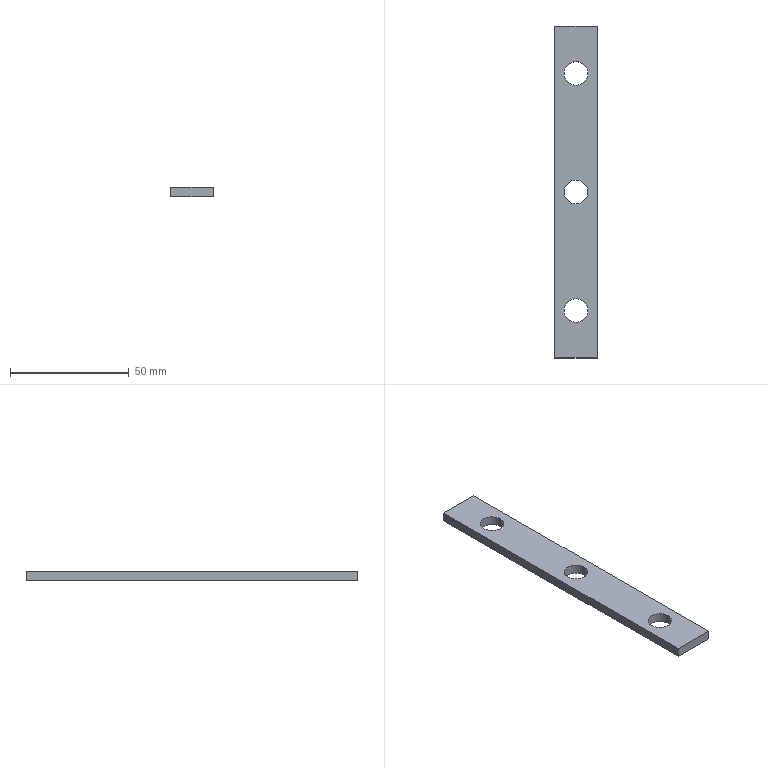Part | SolidWorks | features Extrusion 1 | 1 solid | 12 faces | box 18 x 140 x 4 mm | volume 9138 mm3 | cylinder 6 | plane 6 | commonest cylinder face diameters 10 x6
STEP:
#1=CARTESIAN_POINT('',(-5.,-50.,4.));
#2=VERTEX_POINT('',#1);
#3=CARTESIAN_POINT('',(5.,-50.,4.));
#4=VERTEX_POINT('',#3);
#5=CARTESIAN_POINT('',(0.,-50.,4.));
#6=DIRECTION('',(0.,0.,1.));
#7=DIRECTION('',(1.,0.,0.));
#8=AXIS2_PLACEMENT_3D('',#5,#6,#7);
#9=CIRCLE('',#8,5.);
#10=EDGE_CURVE('',#2,#4,#9,.T.);
#11=ORIENTED_EDGE('',*,*,#10,.T.);
#12=CARTESIAN_POINT('',(5.,-50.,0.));
#13=VERTEX_POINT('',#12);
#14=CARTESIAN_POINT('',(5.,-50.,4.));
#15=DIRECTION('',(0.,0.,-1.));
#16=VECTOR('',#15,1000.);
#17=LINE('',#14,#16);
#18=EDGE_CURVE('',#4,#13,#17,.T.);
#19=ORIENTED_EDGE('',*,*,#18,.T.);
#20=CARTESIAN_POINT('',(-5.,-50.,0.));
#21=VERTEX_POINT('',#20);
#22=CARTESIAN_POINT('',(0.,-50.,0.));
#23=DIRECTION('',(0.,0.,1.));
#24=DIRECTION('',(1.,0.,0.));
#25=AXIS2_PLACEMENT_3D('',#22,#23,#24);
#26=CIRCLE('',#25,5.);
#27=EDGE_CURVE('',#21,#13,#26,.T.);
#28=ORIENTED_EDGE('',*,*,#27,.F.);
#29=CARTESIAN_POINT('',(-5.,-50.,4.));
#30=DIRECTION('',(0.,0.,-1.));
#31=VECTOR('',#30,1000.);
#32=LINE('',#29,#31);
#33=EDGE_CURVE('',#2,#21,#32,.T.);
#34=ORIENTED_EDGE('',*,*,#33,.F.);
#35=EDGE_LOOP('',(#11,#19,#28,#34));
#36=FACE_OUTER_BOUND('',#35,.T.);
#37=CARTESIAN_POINT('',(0.,-50.,4.));
#38=DIRECTION('',(0.,0.,-1.));
#39=DIRECTION('',(-1.,0.,0.));
#40=AXIS2_PLACEMENT_3D('',#37,#38,#39);
#41=CYLINDRICAL_SURFACE('',#40,5.);
#42=ADVANCED_FACE('',(#36),#41,.F.);
#43=CARTESIAN_POINT('',(-5.,0.,4.));
#44=VERTEX_POINT('',#43);
#45=CARTESIAN_POINT('',(5.,0.,4.));
#46=VERTEX_POINT('',#45);
#47=CARTESIAN_POINT('',(0.,0.,4.));
#48=DIRECTION('',(0.,0.,1.));
#49=DIRECTION('',(1.,0.,0.));
#50=AXIS2_PLACEMENT_3D('',#47,#48,#49);
#51=CIRCLE('',#50,5.);
#52=EDGE_CURVE('',#44,#46,#51,.T.);
#53=ORIENTED_EDGE('',*,*,#52,.T.);
#54=CARTESIAN_POINT('',(5.,0.,0.));
#55=VERTEX_POINT('',#54);
#56=CARTESIAN_POINT('',(5.,0.,4.));
#57=DIRECTION('',(0.,0.,-1.));
#58=VECTOR('',#57,1000.);
#59=LINE('',#56,#58);
#60=EDGE_CURVE('',#46,#55,#59,.T.);
#61=ORIENTED_EDGE('',*,*,#60,.T.);
#62=CARTESIAN_POINT('',(-5.,0.,0.));
#63=VERTEX_POINT('',#62);
#64=CARTESIAN_POINT('',(0.,0.,0.));
#65=DIRECTION('',(0.,0.,1.));
#66=DIRECTION('',(1.,0.,0.));
#67=AXIS2_PLACEMENT_3D('',#64,#65,#66);
#68=CIRCLE('',#67,5.);
#69=EDGE_CURVE('',#63,#55,#68,.T.);
#70=ORIENTED_EDGE('',*,*,#69,.F.);
#71=CARTESIAN_POINT('',(-5.,0.,4.));
#72=DIRECTION('',(0.,0.,-1.));
#73=VECTOR('',#72,1000.);
#74=LINE('',#71,#73);
#75=EDGE_CURVE('',#44,#63,#74,.T.);
#76=ORIENTED_EDGE('',*,*,#75,.F.);
#77=EDGE_LOOP('',(#53,#61,#70,#76));
#78=FACE_OUTER_BOUND('',#77,.T.);
#79=CARTESIAN_POINT('',(0.,0.,4.));
#80=DIRECTION('',(0.,0.,-1.));
#81=DIRECTION('',(-1.,0.,0.));
#82=AXIS2_PLACEMENT_3D('',#79,#80,#81);
#83=CYLINDRICAL_SURFACE('',#82,5.);
#84=ADVANCED_FACE('',(#78),#83,.F.);
#85=CARTESIAN_POINT('',(-5.,50.,4.));
#86=VERTEX_POINT('',#85);
#87=CARTESIAN_POINT('',(5.,50.,4.));
#88=VERTEX_POINT('',#87);
#89=CARTESIAN_POINT('',(0.,50.,4.));
#90=DIRECTION('',(0.,0.,1.));
#91=DIRECTION('',(1.,0.,0.));
#92=AXIS2_PLACEMENT_3D('',#89,#90,#91);
#93=CIRCLE('',#92,5.);
#94=EDGE_CURVE('',#86,#88,#93,.T.);
#95=ORIENTED_EDGE('',*,*,#94,.T.);
#96=CARTESIAN_POINT('',(5.,50.,0.));
#97=VERTEX_POINT('',#96);
#98=CARTESIAN_POINT('',(5.,50.,4.));
#99=DIRECTION('',(0.,0.,-1.));
#100=VECTOR('',#99,1000.);
#101=LINE('',#98,#100);
#102=EDGE_CURVE('',#88,#97,#101,.T.);
#103=ORIENTED_EDGE('',*,*,#102,.T.);
#104=CARTESIAN_POINT('',(-5.,50.,0.));
#105=VERTEX_POINT('',#104);
#106=CARTESIAN_POINT('',(0.,50.,0.));
#107=DIRECTION('',(0.,0.,1.));
#108=DIRECTION('',(1.,0.,0.));
#109=AXIS2_PLACEMENT_3D('',#106,#107,#108);
#110=CIRCLE('',#109,5.);
#111=EDGE_CURVE('',#105,#97,#110,.T.);
#112=ORIENTED_EDGE('',*,*,#111,.F.);
#113=CARTESIAN_POINT('',(-5.,50.,4.));
#114=DIRECTION('',(0.,0.,-1.));
#115=VECTOR('',#114,1000.);
#116=LINE('',#113,#115);
#117=EDGE_CURVE('',#86,#105,#116,.T.);
#118=ORIENTED_EDGE('',*,*,#117,.F.);
#119=EDGE_LOOP('',(#95,#103,#112,#118));
#120=FACE_OUTER_BOUND('',#119,.T.);
#121=CARTESIAN_POINT('',(0.,50.,4.));
#122=DIRECTION('',(0.,0.,-1.));
#123=DIRECTION('',(-1.,0.,0.));
#124=AXIS2_PLACEMENT_3D('',#121,#122,#123);
#125=CYLINDRICAL_SURFACE('',#124,5.);
#126=ADVANCED_FACE('',(#120),#125,.F.);
#127=CARTESIAN_POINT('',(9.,-70.,4.));
#128=VERTEX_POINT('',#127);
#129=CARTESIAN_POINT('',(9.,70.,4.));
#130=VERTEX_POINT('',#129);
#131=CARTESIAN_POINT('',(9.,-70.,4.));
#132=DIRECTION('',(0.,1.,0.));
#133=VECTOR('',#132,1000.);
#134=LINE('',#131,#133);
#135=EDGE_CURVE('',#128,#130,#134,.T.);
#136=ORIENTED_EDGE('',*,*,#135,.T.);
#137=CARTESIAN_POINT('',(-9.,70.,4.));
#138=VERTEX_POINT('',#137);
#139=CARTESIAN_POINT('',(-9.,70.,4.));
#140=DIRECTION('',(-1.,0.,0.));
#141=VECTOR('',#140,1000.);
#142=LINE('',#139,#141);
#143=EDGE_CURVE('',#130,#138,#142,.T.);
#144=ORIENTED_EDGE('',*,*,#143,.T.);
#145=CARTESIAN_POINT('',(-9.,-70.,4.));
#146=VERTEX_POINT('',#145);
#147=CARTESIAN_POINT('',(-9.,-70.,4.));
#148=DIRECTION('',(0.,-1.,0.));
#149=VECTOR('',#148,1000.);
#150=LINE('',#147,#149);
#151=EDGE_CURVE('',#138,#146,#150,.T.);
#152=ORIENTED_EDGE('',*,*,#151,.T.);
#153=CARTESIAN_POINT('',(-9.,-70.,4.));
#154=DIRECTION('',(1.,0.,0.));
#155=VECTOR('',#154,1000.);
#156=LINE('',#153,#155);
#157=EDGE_CURVE('',#146,#128,#156,.T.);
#158=ORIENTED_EDGE('',*,*,#157,.T.);
#159=EDGE_LOOP('',(#136,#144,#152,#158));
#160=FACE_OUTER_BOUND('',#159,.T.);
#161=ORIENTED_EDGE('',*,*,#94,.F.);
#162=CARTESIAN_POINT('',(0.,50.,4.));
#163=DIRECTION('',(0.,0.,1.));
#164=DIRECTION('',(1.,0.,0.));
#165=AXIS2_PLACEMENT_3D('',#162,#163,#164);
#166=CIRCLE('',#165,5.);
#167=EDGE_CURVE('',#88,#86,#166,.T.);
#168=ORIENTED_EDGE('',*,*,#167,.F.);
#169=EDGE_LOOP('',(#161,#168));
#170=FACE_BOUND('',#169,.T.);
#171=ORIENTED_EDGE('',*,*,#52,.F.);
#172=CARTESIAN_POINT('',(0.,0.,4.));
#173=DIRECTION('',(0.,0.,1.));
#174=DIRECTION('',(1.,0.,0.));
#175=AXIS2_PLACEMENT_3D('',#172,#173,#174);
#176=CIRCLE('',#175,5.);
#177=EDGE_CURVE('',#46,#44,#176,.T.);
#178=ORIENTED_EDGE('',*,*,#177,.F.);
#179=EDGE_LOOP('',(#171,#178));
#180=FACE_BOUND('',#179,.T.);
#181=ORIENTED_EDGE('',*,*,#10,.F.);
#182=CARTESIAN_POINT('',(0.,-50.,4.));
#183=DIRECTION('',(0.,0.,1.));
#184=DIRECTION('',(1.,0.,0.));
#185=AXIS2_PLACEMENT_3D('',#182,#183,#184);
#186=CIRCLE('',#185,5.);
#187=EDGE_CURVE('',#4,#2,#186,.T.);
#188=ORIENTED_EDGE('',*,*,#187,.F.);
#189=EDGE_LOOP('',(#181,#188));
#190=FACE_BOUND('',#189,.T.);
#191=CARTESIAN_POINT('',(0.,0.,4.));
#192=DIRECTION('',(0.,0.,-1.));
#193=DIRECTION('',(-1.,0.,0.));
#194=AXIS2_PLACEMENT_3D('',#191,#192,#193);
#195=PLANE('',#194);
#196=ADVANCED_FACE('',(#160,#170,#180,#190),#195,.F.);
#197=ORIENTED_EDGE('',*,*,#69,.T.);
#198=CARTESIAN_POINT('',(0.,0.,0.));
#199=DIRECTION('',(0.,0.,1.));
#200=DIRECTION('',(1.,0.,0.));
#201=AXIS2_PLACEMENT_3D('',#198,#199,#200);
#202=CIRCLE('',#201,5.);
#203=EDGE_CURVE('',#55,#63,#202,.T.);
#204=ORIENTED_EDGE('',*,*,#203,.T.);
#205=EDGE_LOOP('',(#197,#204));
#206=FACE_BOUND('',#205,.T.);
#207=CARTESIAN_POINT('',(9.,-70.,0.));
#208=VERTEX_POINT('',#207);
#209=CARTESIAN_POINT('',(9.,70.,0.));
#210=VERTEX_POINT('',#209);
#211=CARTESIAN_POINT('',(9.,-70.,0.));
#212=DIRECTION('',(0.,1.,0.));
#213=VECTOR('',#212,1000.);
#214=LINE('',#211,#213);
#215=EDGE_CURVE('',#208,#210,#214,.T.);
#216=ORIENTED_EDGE('',*,*,#215,.F.);
#217=CARTESIAN_POINT('',(-9.,-70.,0.));
#218=VERTEX_POINT('',#217);
#219=CARTESIAN_POINT('',(-9.,-70.,0.));
#220=DIRECTION('',(1.,0.,0.));
#221=VECTOR('',#220,1000.);
#222=LINE('',#219,#221);
#223=EDGE_CURVE('',#218,#208,#222,.T.);
#224=ORIENTED_EDGE('',*,*,#223,.F.);
#225=CARTESIAN_POINT('',(-9.,70.,0.));
#226=VERTEX_POINT('',#225);
#227=CARTESIAN_POINT('',(-9.,-70.,0.));
#228=DIRECTION('',(0.,-1.,0.));
#229=VECTOR('',#228,1000.);
#230=LINE('',#227,#229);
#231=EDGE_CURVE('',#226,#218,#230,.T.);
#232=ORIENTED_EDGE('',*,*,#231,.F.);
#233=CARTESIAN_POINT('',(-9.,70.,0.));
#234=DIRECTION('',(-1.,0.,0.));
#235=VECTOR('',#234,1000.);
#236=LINE('',#233,#235);
#237=EDGE_CURVE('',#210,#226,#236,.T.);
#238=ORIENTED_EDGE('',*,*,#237,.F.);
#239=EDGE_LOOP('',(#216,#224,#232,#238));
#240=FACE_OUTER_BOUND('',#239,.T.);
#241=ORIENTED_EDGE('',*,*,#111,.T.);
#242=CARTESIAN_POINT('',(0.,50.,0.));
#243=DIRECTION('',(0.,0.,1.));
#244=DIRECTION('',(1.,0.,0.));
#245=AXIS2_PLACEMENT_3D('',#242,#243,#244);
#246=CIRCLE('',#245,5.);
#247=EDGE_CURVE('',#97,#105,#246,.T.);
#248=ORIENTED_EDGE('',*,*,#247,.T.);
#249=EDGE_LOOP('',(#241,#248));
#250=FACE_BOUND('',#249,.T.);
#251=ORIENTED_EDGE('',*,*,#27,.T.);
#252=CARTESIAN_POINT('',(0.,-50.,0.));
#253=DIRECTION('',(0.,0.,1.));
#254=DIRECTION('',(1.,0.,0.));
#255=AXIS2_PLACEMENT_3D('',#252,#253,#254);
#256=CIRCLE('',#255,5.);
#257=EDGE_CURVE('',#13,#21,#256,.T.);
#258=ORIENTED_EDGE('',*,*,#257,.T.);
#259=EDGE_LOOP('',(#251,#258));
#260=FACE_BOUND('',#259,.T.);
#261=CARTESIAN_POINT('',(0.,0.,0.));
#262=DIRECTION('',(0.,0.,-1.));
#263=DIRECTION('',(-1.,0.,0.));
#264=AXIS2_PLACEMENT_3D('',#261,#262,#263);
#265=PLANE('',#264);
#266=ADVANCED_FACE('',(#206,#240,#250,#260),#265,.T.);
#267=ORIENTED_EDGE('',*,*,#215,.T.);
#268=CARTESIAN_POINT('',(9.,70.,4.));
#269=DIRECTION('',(0.,0.,-1.));
#270=VECTOR('',#269,1000.);
#271=LINE('',#268,#270);
#272=EDGE_CURVE('',#130,#210,#271,.T.);
#273=ORIENTED_EDGE('',*,*,#272,.F.);
#274=ORIENTED_EDGE('',*,*,#135,.F.);
#275=CARTESIAN_POINT('',(9.,-70.,4.));
#276=DIRECTION('',(0.,0.,-1.));
#277=VECTOR('',#276,1000.);
#278=LINE('',#275,#277);
#279=EDGE_CURVE('',#128,#208,#278,.T.);
#280=ORIENTED_EDGE('',*,*,#279,.T.);
#281=EDGE_LOOP('',(#267,#273,#274,#280));
#282=FACE_OUTER_BOUND('',#281,.T.);
#283=CARTESIAN_POINT('',(9.,-70.,4.));
#284=DIRECTION('',(-1.,0.,0.));
#285=DIRECTION('',(0.,0.,1.));
#286=AXIS2_PLACEMENT_3D('',#283,#284,#285);
#287=PLANE('',#286);
#288=ADVANCED_FACE('',(#282),#287,.F.);
#289=ORIENTED_EDGE('',*,*,#237,.T.);
#290=CARTESIAN_POINT('',(-9.,70.,4.));
#291=DIRECTION('',(0.,0.,-1.));
#292=VECTOR('',#291,1000.);
#293=LINE('',#290,#292);
#294=EDGE_CURVE('',#138,#226,#293,.T.);
#295=ORIENTED_EDGE('',*,*,#294,.F.);
#296=ORIENTED_EDGE('',*,*,#143,.F.);
#297=ORIENTED_EDGE('',*,*,#272,.T.);
#298=EDGE_LOOP('',(#289,#295,#296,#297));
#299=FACE_OUTER_BOUND('',#298,.T.);
#300=CARTESIAN_POINT('',(-9.,70.,4.));
#301=DIRECTION('',(0.,-1.,0.));
#302=DIRECTION('',(0.,0.,-1.));
#303=AXIS2_PLACEMENT_3D('',#300,#301,#302);
#304=PLANE('',#303);
#305=ADVANCED_FACE('',(#299),#304,.F.);
#306=ORIENTED_EDGE('',*,*,#231,.T.);
#307=CARTESIAN_POINT('',(-9.,-70.,4.));
#308=DIRECTION('',(0.,0.,-1.));
#309=VECTOR('',#308,1000.);
#310=LINE('',#307,#309);
#311=EDGE_CURVE('',#146,#218,#310,.T.);
#312=ORIENTED_EDGE('',*,*,#311,.F.);
#313=ORIENTED_EDGE('',*,*,#151,.F.);
#314=ORIENTED_EDGE('',*,*,#294,.T.);
#315=EDGE_LOOP('',(#306,#312,#313,#314));
#316=FACE_OUTER_BOUND('',#315,.T.);
#317=CARTESIAN_POINT('',(-9.,-70.,4.));
#318=DIRECTION('',(1.,0.,0.));
#319=DIRECTION('',(0.,0.,-1.));
#320=AXIS2_PLACEMENT_3D('',#317,#318,#319);
#321=PLANE('',#320);
#322=ADVANCED_FACE('',(#316),#321,.F.);
#323=ORIENTED_EDGE('',*,*,#223,.T.);
#324=ORIENTED_EDGE('',*,*,#279,.F.);
#325=ORIENTED_EDGE('',*,*,#157,.F.);
#326=ORIENTED_EDGE('',*,*,#311,.T.);
#327=EDGE_LOOP('',(#323,#324,#325,#326));
#328=FACE_OUTER_BOUND('',#327,.T.);
#329=CARTESIAN_POINT('',(-9.,-70.,4.));
#330=DIRECTION('',(0.,1.,0.));
#331=DIRECTION('',(0.,0.,1.));
#332=AXIS2_PLACEMENT_3D('',#329,#330,#331);
#333=PLANE('',#332);
#334=ADVANCED_FACE('',(#328),#333,.F.);
#335=ORIENTED_EDGE('',*,*,#102,.F.);
#336=ORIENTED_EDGE('',*,*,#167,.T.);
#337=ORIENTED_EDGE('',*,*,#117,.T.);
#338=ORIENTED_EDGE('',*,*,#247,.F.);
#339=EDGE_LOOP('',(#335,#336,#337,#338));
#340=FACE_OUTER_BOUND('',#339,.T.);
#341=CARTESIAN_POINT('',(0.,50.,4.));
#342=DIRECTION('',(0.,0.,-1.));
#343=DIRECTION('',(-1.,0.,0.));
#344=AXIS2_PLACEMENT_3D('',#341,#342,#343);
#345=CYLINDRICAL_SURFACE('',#344,5.);
#346=ADVANCED_FACE('',(#340),#345,.F.);
#347=ORIENTED_EDGE('',*,*,#60,.F.);
#348=ORIENTED_EDGE('',*,*,#177,.T.);
#349=ORIENTED_EDGE('',*,*,#75,.T.);
#350=ORIENTED_EDGE('',*,*,#203,.F.);
#351=EDGE_LOOP('',(#347,#348,#349,#350));
#352=FACE_OUTER_BOUND('',#351,.T.);
#353=CARTESIAN_POINT('',(0.,0.,4.));
#354=DIRECTION('',(0.,0.,-1.));
#355=DIRECTION('',(-1.,0.,0.));
#356=AXIS2_PLACEMENT_3D('',#353,#354,#355);
#357=CYLINDRICAL_SURFACE('',#356,5.);
#358=ADVANCED_FACE('',(#352),#357,.F.);
#359=ORIENTED_EDGE('',*,*,#18,.F.);
#360=ORIENTED_EDGE('',*,*,#187,.T.);
#361=ORIENTED_EDGE('',*,*,#33,.T.);
#362=ORIENTED_EDGE('',*,*,#257,.F.);
#363=EDGE_LOOP('',(#359,#360,#361,#362));
#364=FACE_OUTER_BOUND('',#363,.T.);
#365=CARTESIAN_POINT('',(0.,-50.,4.));
#366=DIRECTION('',(0.,0.,-1.));
#367=DIRECTION('',(-1.,0.,0.));
#368=AXIS2_PLACEMENT_3D('',#365,#366,#367);
#369=CYLINDRICAL_SURFACE('',#368,5.);
#370=ADVANCED_FACE('',(#364),#369,.F.);
#371=CLOSED_SHELL('',(#42,#84,#126,#196,#266,#288,#305,#322,#334,#346,#358,#370));
#372=MANIFOLD_SOLID_BREP('',#371);
#373=CARTESIAN_POINT('',(0.,0.,0.));
#374=DIRECTION('',(0.,0.,1.));
#375=DIRECTION('',(1.,0.,0.));
#376=AXIS2_PLACEMENT_3D('',#373,#374,#375);
#377=(LENGTH_UNIT()NAMED_UNIT(*)SI_UNIT(.MILLI.,.METRE.));
#378=UNCERTAINTY_MEASURE_WITH_UNIT(LENGTH_MEASURE(0.00001),#377,'','');
#379=(NAMED_UNIT(*)PLANE_ANGLE_UNIT()SI_UNIT($,.RADIAN.));
#380=(NAMED_UNIT(*)SI_UNIT($,.STERADIAN.)SOLID_ANGLE_UNIT());
#381=(GEOMETRIC_REPRESENTATION_CONTEXT(3)GLOBAL_UNCERTAINTY_ASSIGNED_CONTEXT((#378))GLOBAL_UNIT_ASSIGNED_CONTEXT((#377,#379,#380))REPRESENTATION_CONTEXT('',''));
#382=ADVANCED_BREP_SHAPE_REPRESENTATION('',(#372,#376),#381);